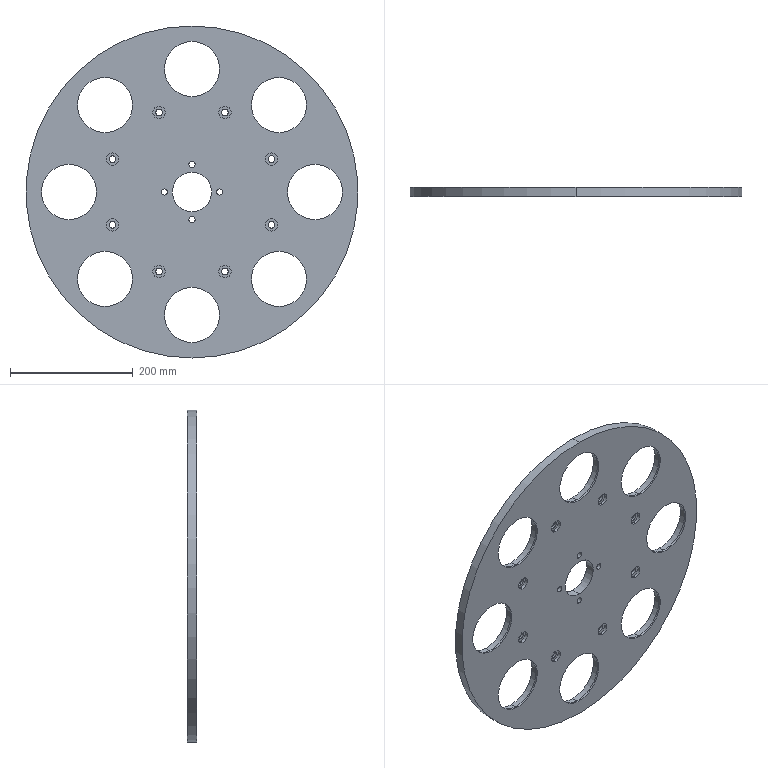Part | SolidWorks | features BaseBody 1 | 1 solid | 110 faces | box 540 x 15 x 540 mm | volume 2513615 mm3 | cylinder 76 | plane 18 | cone 16 | commonest cylinder face diameters 11 x16 20 x16 89.8 x16 95.7 x16 10 x8 64 x2